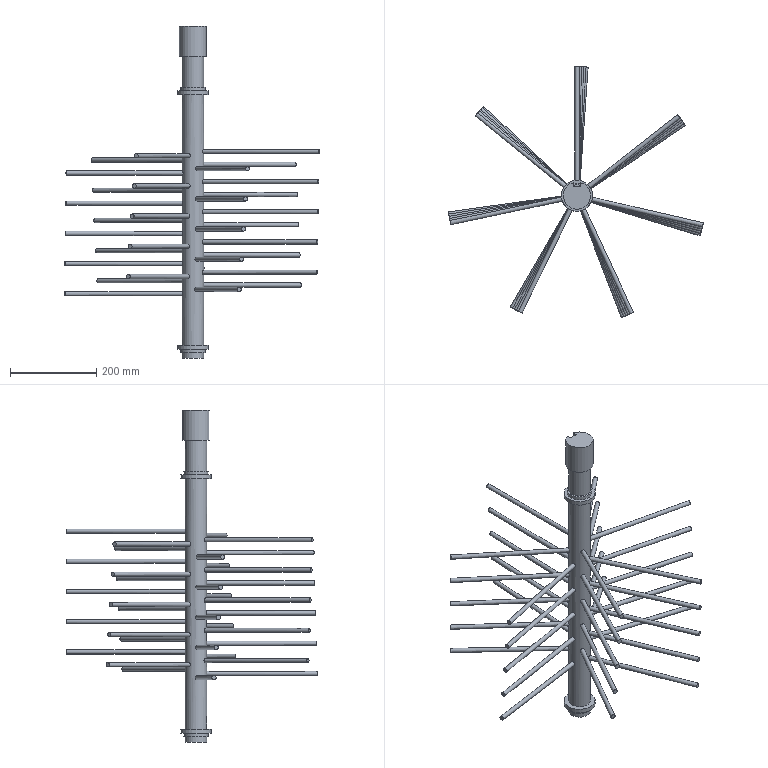Part | NX | 1 solid | 91 faces | box 591.212 x 581.908 x 770 mm | volume 2385468 mm3 | plane 48 | cylinder 43 | commonest cylinder face diameters 10 x35 50 x3 57.334 x2 72 x2 63 x1